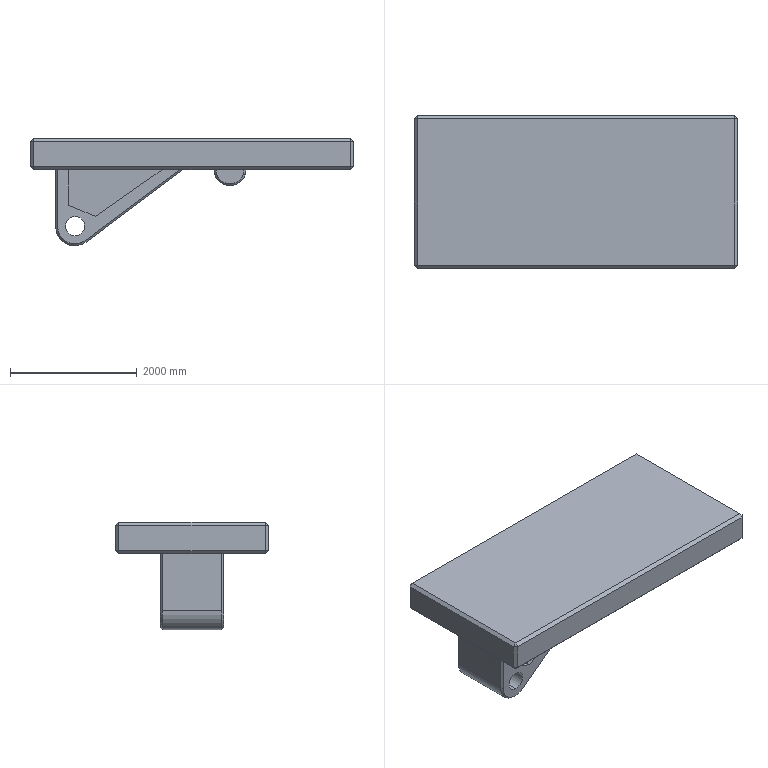Part | SolidWorks | features ICE 6, Chamfer 3, MirrorPattern 2, Extrusion 1, Fillet 1 | 1 solid | 66 faces | box 5102 x 2411 x 1700 mm | volume 7041996598 mm3 | plane 51 | cylinder 9 | cone 6 | commonest cylinder face diameters 500 x3 250 x2 300 x2 600 x2